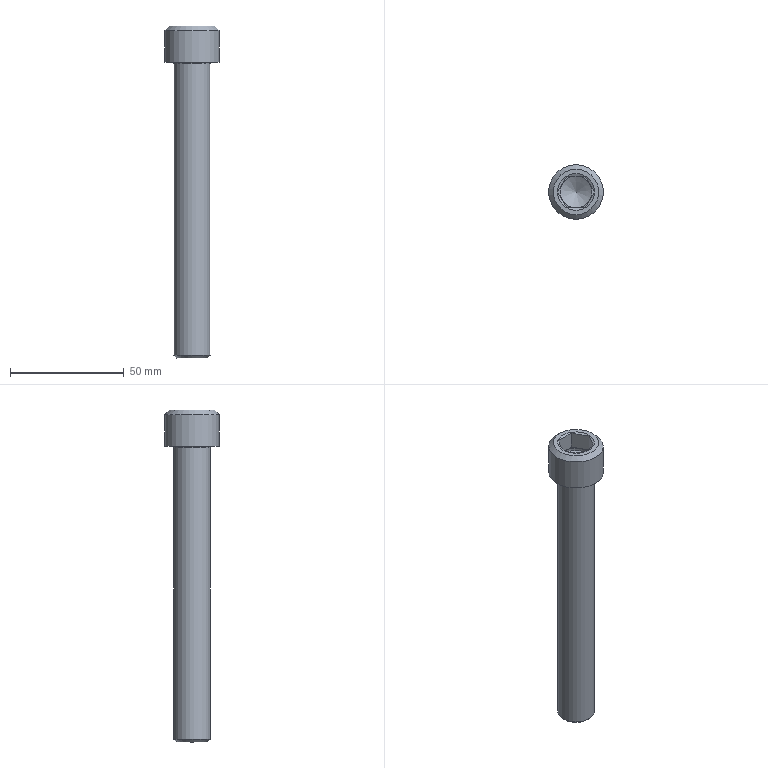Part | NX | features MAIN_BODY 2 | 1 solid | 20 faces | box 24 x 24 x 146 mm | volume 31440 mm3 | plane 11 | cone 5 | cylinder 3 | torus 1 | commonest cylinder face diameters 14 x1 16 x1 24 x1
STEP:
#1=CARTESIAN_POINT('',(635.,-653.001,267.));
#2=VERTEX_POINT('',#1);
#3=CARTESIAN_POINT('',(635.,-665.001,267.));
#4=DIRECTION('',(0.,0.,-1.));
#5=DIRECTION('',(0.,1.,0.));
#6=AXIS2_PLACEMENT_3D('',#3,#4,#5);
#7=CIRCLE('',#6,12.);
#8=EDGE_CURVE('',#2,#2,#7,.F.);
#9=ORIENTED_EDGE('',*,*,#8,.F.);
#10=EDGE_LOOP('',(#9));
#11=FACE_BOUND('',#10,.T.);
#12=CARTESIAN_POINT('',(635.,-677.001,253.));
#13=VERTEX_POINT('',#12);
#14=CARTESIAN_POINT('',(635.,-665.001,253.));
#15=DIRECTION('',(0.,0.,1.));
#16=DIRECTION('',(0.,-1.,0.));
#17=AXIS2_PLACEMENT_3D('',#14,#15,#16);
#18=CIRCLE('',#17,12.);
#19=EDGE_CURVE('',#13,#13,#18,.T.);
#20=ORIENTED_EDGE('',*,*,#19,.T.);
#21=EDGE_LOOP('',(#20));
#22=FACE_BOUND('',#21,.T.);
#23=CARTESIAN_POINT('',(635.,-665.001,261.));
#24=DIRECTION('',(0.,0.,1.));
#25=DIRECTION('',(0.,1.,0.));
#26=AXIS2_PLACEMENT_3D('',#23,#24,#25);
#27=CYLINDRICAL_SURFACE('',#26,12.);
#28=ADVANCED_FACE('',(#11,#22),#27,.T.);
#29=CARTESIAN_POINT('',(643.1,-665.001,269.));
#30=VERTEX_POINT('',#29);
#31=CARTESIAN_POINT('',(626.9,-665.001,269.));
#32=VERTEX_POINT('',#31);
#33=CARTESIAN_POINT('',(635.,-665.001,269.));
#34=DIRECTION('',(0.,0.,-1.));
#35=DIRECTION('',(0.,1.,0.));
#36=AXIS2_PLACEMENT_3D('',#33,#34,#35);
#37=CIRCLE('',#36,8.1);
#38=EDGE_CURVE('',#30,#32,#37,.T.);
#39=ORIENTED_EDGE('',*,*,#38,.T.);
#40=CARTESIAN_POINT('',(635.,-665.001,269.));
#41=DIRECTION('',(0.,0.,1.));
#42=DIRECTION('',(0.,-1.,0.));
#43=AXIS2_PLACEMENT_3D('',#40,#41,#42);
#44=CIRCLE('',#43,8.1);
#45=EDGE_CURVE('',#30,#32,#44,.T.);
#46=ORIENTED_EDGE('',*,*,#45,.F.);
#47=EDGE_LOOP('',(#39,#46));
#48=FACE_BOUND('',#47,.T.);
#49=CARTESIAN_POINT('',(635.,-655.001,269.));
#50=VERTEX_POINT('',#49);
#51=CARTESIAN_POINT('',(635.,-665.001,269.));
#52=DIRECTION('',(0.,0.,-1.));
#53=DIRECTION('',(0.,1.,0.));
#54=AXIS2_PLACEMENT_3D('',#51,#52,#53);
#55=CIRCLE('',#54,10.);
#56=EDGE_CURVE('',#50,#50,#55,.T.);
#57=ORIENTED_EDGE('',*,*,#56,.F.);
#58=EDGE_LOOP('',(#57));
#59=FACE_BOUND('',#58,.T.);
#60=CARTESIAN_POINT('',(635.,-665.001,269.));
#61=DIRECTION('',(0.,0.,1.));
#62=DIRECTION('',(0.,1.,0.));
#63=AXIS2_PLACEMENT_3D('',#60,#61,#62);
#64=PLANE('',#63);
#65=ADVANCED_FACE('',(#48,#59),#64,.T.);
#66=CARTESIAN_POINT('',(635.,-673.601,253.));
#67=VERTEX_POINT('',#66);
#68=CARTESIAN_POINT('',(635.,-665.001,253.));
#69=DIRECTION('',(0.,0.,1.));
#70=DIRECTION('',(0.,-1.,0.));
#71=AXIS2_PLACEMENT_3D('',#68,#69,#70);
#72=CIRCLE('',#71,8.6);
#73=EDGE_CURVE('',#67,#67,#72,.F.);
#74=ORIENTED_EDGE('',*,*,#73,.F.);
#75=EDGE_LOOP('',(#74));
#76=FACE_BOUND('',#75,.T.);
#77=ORIENTED_EDGE('',*,*,#19,.F.);
#78=EDGE_LOOP('',(#77));
#79=FACE_BOUND('',#78,.T.);
#80=CARTESIAN_POINT('',(635.,-665.001,253.));
#81=DIRECTION('',(0.,0.,-1.));
#82=DIRECTION('',(0.,-1.,0.));
#83=AXIS2_PLACEMENT_3D('',#80,#81,#82);
#84=PLANE('',#83);
#85=ADVANCED_FACE('',(#76,#79),#84,.T.);
#86=CARTESIAN_POINT('',(635.,-671.801,123.));
#87=VERTEX_POINT('',#86);
#88=CARTESIAN_POINT('',(635.,-665.001,123.));
#89=DIRECTION('',(0.,0.,1.));
#90=DIRECTION('',(0.,-1.,0.));
#91=AXIS2_PLACEMENT_3D('',#88,#89,#90);
#92=CIRCLE('',#91,6.8);
#93=EDGE_CURVE('',#87,#87,#92,.T.);
#94=ORIENTED_EDGE('',*,*,#93,.F.);
#95=EDGE_LOOP('',(#94));
#96=FACE_BOUND('',#95,.T.);
#97=CARTESIAN_POINT('',(635.,-665.001,123.));
#98=DIRECTION('',(0.,0.,-1.));
#99=DIRECTION('',(0.,-1.,0.));
#100=AXIS2_PLACEMENT_3D('',#97,#98,#99);
#101=PLANE('',#100);
#102=ADVANCED_FACE('',(#96),#101,.T.);
#103=CARTESIAN_POINT('',(635.,-673.001,252.4));
#104=VERTEX_POINT('',#103);
#105=CARTESIAN_POINT('',(635.,-665.001,252.4));
#106=DIRECTION('',(0.,0.,1.));
#107=DIRECTION('',(0.,-1.,0.));
#108=AXIS2_PLACEMENT_3D('',#105,#106,#107);
#109=CIRCLE('',#108,8.);
#110=EDGE_CURVE('',#104,#104,#109,.T.);
#111=ORIENTED_EDGE('',*,*,#110,.F.);
#112=EDGE_LOOP('',(#111));
#113=FACE_BOUND('',#112,.T.);
#114=CARTESIAN_POINT('',(635.,-673.001,124.2));
#115=VERTEX_POINT('',#114);
#116=CARTESIAN_POINT('',(635.,-665.001,124.2));
#117=DIRECTION('',(0.,0.,1.));
#118=DIRECTION('',(0.,-1.,0.));
#119=AXIS2_PLACEMENT_3D('',#116,#117,#118);
#120=CIRCLE('',#119,8.);
#121=EDGE_CURVE('',#115,#115,#120,.F.);
#122=ORIENTED_EDGE('',*,*,#121,.F.);
#123=EDGE_LOOP('',(#122));
#124=FACE_BOUND('',#123,.T.);
#125=CARTESIAN_POINT('',(635.,-665.001,253.));
#126=DIRECTION('',(0.,0.,-1.));
#127=DIRECTION('',(0.,-1.,0.));
#128=AXIS2_PLACEMENT_3D('',#125,#126,#127);
#129=CYLINDRICAL_SURFACE('',#128,8.);
#130=ADVANCED_FACE('',(#113,#124),#129,.T.);
#131=ORIENTED_EDGE('',*,*,#121,.T.);
#132=EDGE_LOOP('',(#131));
#133=FACE_BOUND('',#132,.T.);
#134=ORIENTED_EDGE('',*,*,#93,.T.);
#135=EDGE_LOOP('',(#134));
#136=FACE_BOUND('',#135,.T.);
#137=CARTESIAN_POINT('',(635.,-665.001,123.));
#138=DIRECTION('',(0.,0.,1.));
#139=DIRECTION('',(0.,1.,0.));
#140=AXIS2_PLACEMENT_3D('',#137,#138,#139);
#141=CONICAL_SURFACE('',#140,6.8,0.7854);
#142=ADVANCED_FACE('',(#133,#136),#141,.T.);
#143=ORIENTED_EDGE('',*,*,#8,.T.);
#144=EDGE_LOOP('',(#143));
#145=FACE_BOUND('',#144,.T.);
#146=ORIENTED_EDGE('',*,*,#56,.T.);
#147=EDGE_LOOP('',(#146));
#148=FACE_BOUND('',#147,.T.);
#149=CARTESIAN_POINT('',(635.,-665.001,269.));
#150=DIRECTION('',(0.,0.,-1.));
#151=DIRECTION('',(0.,-1.,0.));
#152=AXIS2_PLACEMENT_3D('',#149,#150,#151);
#153=CONICAL_SURFACE('',#152,10.,0.7854);
#154=ADVANCED_FACE('',(#145,#148),#153,.T.);
#155=ORIENTED_EDGE('',*,*,#73,.T.);
#156=EDGE_LOOP('',(#155));
#157=FACE_BOUND('',#156,.T.);
#158=ORIENTED_EDGE('',*,*,#110,.T.);
#159=EDGE_LOOP('',(#158));
#160=FACE_BOUND('',#159,.T.);
#161=CARTESIAN_POINT('',(635.,-665.001,252.4));
#162=DIRECTION('',(0.,0.,-1.));
#163=DIRECTION('',(0.,-1.,0.));
#164=AXIS2_PLACEMENT_3D('',#161,#162,#163);
#165=TOROIDAL_SURFACE('',#164,8.6,0.6);
#166=ADVANCED_FACE('',(#157,#160),#165,.F.);
#167=CARTESIAN_POINT('',(630.941,-658.001,268.995));
#168=VERTEX_POINT('',#167);
#169=CARTESIAN_POINT('',(626.9,-665.001,269.));
#170=CARTESIAN_POINT('',(627.56,-663.858,268.619));
#171=CARTESIAN_POINT('',(628.913,-661.514,268.13));
#172=CARTESIAN_POINT('',(630.281,-659.146,268.615));
#173=CARTESIAN_POINT('',(630.941,-658.001,268.995));
#174=B_SPLINE_CURVE_WITH_KNOTS('',3,(#169,#170,#171,#172,#173),.UNSPECIFIED.,.F.,.F.,(4,1,4),(0.000000238,0.004082,0.008163),.UNSPECIFIED.);
#175=EDGE_CURVE('',#32,#168,#174,.T.);
#176=ORIENTED_EDGE('',*,*,#175,.T.);
#177=CARTESIAN_POINT('',(639.059,-658.001,268.995));
#178=VERTEX_POINT('',#177);
#179=CARTESIAN_POINT('',(630.941,-658.001,268.995));
#180=CARTESIAN_POINT('',(632.26,-658.001,268.613));
#181=CARTESIAN_POINT('',(634.999,-658.001,268.116));
#182=CARTESIAN_POINT('',(637.747,-658.001,268.615));
#183=CARTESIAN_POINT('',(639.059,-658.001,268.995));
#184=B_SPLINE_CURVE_WITH_KNOTS('',3,(#179,#180,#181,#182,#183),.UNSPECIFIED.,.F.,.F.,(4,1,4),(0.00695,0.01105,0.01516),.UNSPECIFIED.);
#185=EDGE_CURVE('',#168,#178,#184,.T.);
#186=ORIENTED_EDGE('',*,*,#185,.T.);
#187=CARTESIAN_POINT('',(639.059,-658.001,268.995));
#188=CARTESIAN_POINT('',(639.719,-659.144,268.615));
#189=CARTESIAN_POINT('',(641.072,-661.488,268.13));
#190=CARTESIAN_POINT('',(642.439,-663.857,268.619));
#191=CARTESIAN_POINT('',(643.1,-665.001,269.));
#192=B_SPLINE_CURVE_WITH_KNOTS('',3,(#187,#188,#189,#190,#191),.UNSPECIFIED.,.F.,.F.,(4,1,4),(0.000000238,0.004082,0.008163),.UNSPECIFIED.);
#193=EDGE_CURVE('',#178,#30,#192,.T.);
#194=ORIENTED_EDGE('',*,*,#193,.T.);
#195=ORIENTED_EDGE('',*,*,#45,.T.);
#196=EDGE_LOOP('',(#176,#186,#194,#195));
#197=FACE_BOUND('',#196,.T.);
#198=CARTESIAN_POINT('',(635.,-665.001,264.323));
#199=DIRECTION('',(0.,0.,1.));
#200=DIRECTION('',(0.,1.,0.));
#201=AXIS2_PLACEMENT_3D('',#198,#199,#200);
#202=CONICAL_SURFACE('',#201,0.,1.047);
#203=ADVANCED_FACE('',(#197),#202,.F.);
#204=CARTESIAN_POINT('',(639.059,-672.001,268.995));
#205=VERTEX_POINT('',#204);
#206=CARTESIAN_POINT('',(630.941,-672.001,268.995));
#207=VERTEX_POINT('',#206);
#208=CARTESIAN_POINT('',(630.941,-672.001,268.995));
#209=CARTESIAN_POINT('',(632.26,-672.001,268.613));
#210=CARTESIAN_POINT('',(634.999,-672.001,268.116));
#211=CARTESIAN_POINT('',(637.747,-672.001,268.615));
#212=CARTESIAN_POINT('',(639.059,-672.001,268.995));
#213=B_SPLINE_CURVE_WITH_KNOTS('',3,(#208,#209,#210,#211,#212),.UNSPECIFIED.,.F.,.F.,(4,1,4),(0.00695,0.01105,0.01516),.UNSPECIFIED.);
#214=EDGE_CURVE('',#205,#207,#213,.F.);
#215=ORIENTED_EDGE('',*,*,#214,.T.);
#216=CARTESIAN_POINT('',(630.941,-672.001,268.995));
#217=CARTESIAN_POINT('',(630.281,-670.858,268.615));
#218=CARTESIAN_POINT('',(628.928,-668.513,268.13));
#219=CARTESIAN_POINT('',(627.561,-666.145,268.619));
#220=CARTESIAN_POINT('',(626.9,-665.001,269.));
#221=B_SPLINE_CURVE_WITH_KNOTS('',3,(#216,#217,#218,#219,#220),.UNSPECIFIED.,.F.,.F.,(4,1,4),(0.000000238,0.004082,0.008163),.UNSPECIFIED.);
#222=EDGE_CURVE('',#207,#32,#221,.T.);
#223=ORIENTED_EDGE('',*,*,#222,.T.);
#224=ORIENTED_EDGE('',*,*,#38,.F.);
#225=CARTESIAN_POINT('',(639.059,-672.001,268.995));
#226=CARTESIAN_POINT('',(639.719,-670.858,268.615));
#227=CARTESIAN_POINT('',(641.072,-668.513,268.13));
#228=CARTESIAN_POINT('',(642.439,-666.145,268.619));
#229=CARTESIAN_POINT('',(643.1,-665.001,269.));
#230=B_SPLINE_CURVE_WITH_KNOTS('',3,(#225,#226,#227,#228,#229),.UNSPECIFIED.,.F.,.F.,(4,1,4),(0.000000238,0.004082,0.008163),.UNSPECIFIED.);
#231=EDGE_CURVE('',#205,#30,#230,.T.);
#232=ORIENTED_EDGE('',*,*,#231,.F.);
#233=EDGE_LOOP('',(#215,#223,#224,#232));
#234=FACE_BOUND('',#233,.T.);
#235=CARTESIAN_POINT('',(635.,-665.001,264.323));
#236=DIRECTION('',(0.,0.,1.));
#237=DIRECTION('',(0.,1.,0.));
#238=AXIS2_PLACEMENT_3D('',#235,#236,#237);
#239=CONICAL_SURFACE('',#238,0.,1.047);
#240=ADVANCED_FACE('',(#234),#239,.F.);
#241=CARTESIAN_POINT('',(635.,-672.001,259.8));
#242=VERTEX_POINT('',#241);
#243=CARTESIAN_POINT('',(635.,-665.001,259.8));
#244=DIRECTION('',(0.,0.,1.));
#245=DIRECTION('',(0.,-1.,0.));
#246=AXIS2_PLACEMENT_3D('',#243,#244,#245);
#247=CIRCLE('',#246,7.);
#248=EDGE_CURVE('',#242,#242,#247,.T.);
#249=ORIENTED_EDGE('',*,*,#248,.T.);
#250=EDGE_LOOP('',(#249));
#251=FACE_BOUND('',#250,.T.);
#252=CARTESIAN_POINT('',(635.,-665.001,255.759));
#253=VERTEX_POINT('',#252);
#254=VERTEX_LOOP('',#253);
#255=FACE_BOUND('',#254,.T.);
#256=CARTESIAN_POINT('',(635.,-665.001,259.8));
#257=DIRECTION('',(0.,0.,1.));
#258=DIRECTION('',(0.,1.,0.));
#259=AXIS2_PLACEMENT_3D('',#256,#257,#258);
#260=CONICAL_SURFACE('',#259,7.,1.047);
#261=ADVANCED_FACE('',(#251,#255),#260,.F.);
#262=ORIENTED_EDGE('',*,*,#248,.F.);
#263=EDGE_LOOP('',(#262));
#264=FACE_BOUND('',#263,.T.);
#265=CARTESIAN_POINT('',(635.,-672.001,261.));
#266=VERTEX_POINT('',#265);
#267=CARTESIAN_POINT('',(635.,-658.001,261.));
#268=VERTEX_POINT('',#267);
#269=CARTESIAN_POINT('',(635.,-665.001,261.));
#270=DIRECTION('',(0.,0.,1.));
#271=DIRECTION('',(0.,-1.,0.));
#272=AXIS2_PLACEMENT_3D('',#269,#270,#271);
#273=CIRCLE('',#272,7.);
#274=EDGE_CURVE('',#266,#268,#273,.T.);
#275=ORIENTED_EDGE('',*,*,#274,.T.);
#276=CARTESIAN_POINT('',(635.,-665.001,261.));
#277=DIRECTION('',(0.,0.,1.));
#278=DIRECTION('',(0.,-1.,0.));
#279=AXIS2_PLACEMENT_3D('',#276,#277,#278);
#280=CIRCLE('',#279,7.);
#281=EDGE_CURVE('',#268,#266,#280,.T.);
#282=ORIENTED_EDGE('',*,*,#281,.T.);
#283=EDGE_LOOP('',(#275,#282));
#284=FACE_BOUND('',#283,.T.);
#285=CARTESIAN_POINT('',(635.,-665.001,261.));
#286=DIRECTION('',(0.,0.,-1.));
#287=DIRECTION('',(0.,-1.,0.));
#288=AXIS2_PLACEMENT_3D('',#285,#286,#287);
#289=CYLINDRICAL_SURFACE('',#288,7.);
#290=ADVANCED_FACE('',(#264,#284),#289,.F.);
#291=CARTESIAN_POINT('',(630.941,-658.001,261.));
#292=VERTEX_POINT('',#291);
#293=CARTESIAN_POINT('',(630.941,-658.001,261.));
#294=DIRECTION('',(1.,0.,0.));
#295=VECTOR('',#294,1000.);
#296=LINE('',#293,#295);
#297=EDGE_CURVE('',#292,#268,#296,.T.);
#298=ORIENTED_EDGE('',*,*,#297,.F.);
#299=CARTESIAN_POINT('',(626.9,-665.001,261.));
#300=VERTEX_POINT('',#299);
#301=CARTESIAN_POINT('',(626.9,-665.001,261.));
#302=DIRECTION('',(0.5,0.866,0.));
#303=VECTOR('',#302,1000.);
#304=LINE('',#301,#303);
#305=EDGE_CURVE('',#300,#292,#304,.T.);
#306=ORIENTED_EDGE('',*,*,#305,.F.);
#307=CARTESIAN_POINT('',(630.941,-672.001,261.));
#308=VERTEX_POINT('',#307);
#309=CARTESIAN_POINT('',(630.941,-672.001,261.));
#310=DIRECTION('',(-0.5,0.866,0.));
#311=VECTOR('',#310,1000.);
#312=LINE('',#309,#311);
#313=EDGE_CURVE('',#308,#300,#312,.T.);
#314=ORIENTED_EDGE('',*,*,#313,.F.);
#315=CARTESIAN_POINT('',(639.059,-672.001,261.));
#316=DIRECTION('',(-1.,0.,0.));
#317=VECTOR('',#316,1000.);
#318=LINE('',#315,#317);
#319=EDGE_CURVE('',#266,#308,#318,.T.);
#320=ORIENTED_EDGE('',*,*,#319,.F.);
#321=ORIENTED_EDGE('',*,*,#281,.F.);
#322=EDGE_LOOP('',(#298,#306,#314,#320,#321));
#323=FACE_BOUND('',#322,.T.);
#324=CARTESIAN_POINT('',(635.,-665.001,261.));
#325=DIRECTION('',(0.,0.,1.));
#326=DIRECTION('',(0.,1.,0.));
#327=AXIS2_PLACEMENT_3D('',#324,#325,#326);
#328=PLANE('',#327);
#329=ADVANCED_FACE('',(#323),#328,.T.);
#330=CARTESIAN_POINT('',(639.059,-672.001,261.));
#331=VERTEX_POINT('',#330);
#332=CARTESIAN_POINT('',(639.059,-672.001,261.));
#333=DIRECTION('',(-1.,0.,0.));
#334=VECTOR('',#333,1000.);
#335=LINE('',#332,#334);
#336=EDGE_CURVE('',#331,#266,#335,.T.);
#337=ORIENTED_EDGE('',*,*,#336,.F.);
#338=CARTESIAN_POINT('',(643.1,-665.001,261.));
#339=VERTEX_POINT('',#338);
#340=CARTESIAN_POINT('',(639.059,-672.001,261.));
#341=DIRECTION('',(0.5,0.866,0.));
#342=VECTOR('',#341,1000.);
#343=LINE('',#340,#342);
#344=EDGE_CURVE('',#331,#339,#343,.T.);
#345=ORIENTED_EDGE('',*,*,#344,.T.);
#346=CARTESIAN_POINT('',(639.059,-658.001,261.));
#347=VERTEX_POINT('',#346);
#348=CARTESIAN_POINT('',(639.059,-658.001,261.));
#349=DIRECTION('',(0.5,-0.866,0.));
#350=VECTOR('',#349,1000.);
#351=LINE('',#348,#350);
#352=EDGE_CURVE('',#347,#339,#351,.T.);
#353=ORIENTED_EDGE('',*,*,#352,.F.);
#354=CARTESIAN_POINT('',(630.941,-658.001,261.));
#355=DIRECTION('',(1.,0.,0.));
#356=VECTOR('',#355,1000.);
#357=LINE('',#354,#356);
#358=EDGE_CURVE('',#268,#347,#357,.T.);
#359=ORIENTED_EDGE('',*,*,#358,.F.);
#360=ORIENTED_EDGE('',*,*,#274,.F.);
#361=EDGE_LOOP('',(#337,#345,#353,#359,#360));
#362=FACE_BOUND('',#361,.T.);
#363=CARTESIAN_POINT('',(635.,-665.001,261.));
#364=DIRECTION('',(0.,0.,1.));
#365=DIRECTION('',(0.,1.,0.));
#366=AXIS2_PLACEMENT_3D('',#363,#364,#365);
#367=PLANE('',#366);
#368=ADVANCED_FACE('',(#362),#367,.T.);
#369=CARTESIAN_POINT('',(639.059,-658.001,261.));
#370=DIRECTION('',(0.,0.,1.));
#371=VECTOR('',#370,1000.);
#372=LINE('',#369,#371);
#373=EDGE_CURVE('',#347,#178,#372,.T.);
#374=ORIENTED_EDGE('',*,*,#373,.F.);
#375=ORIENTED_EDGE('',*,*,#352,.T.);
#376=CARTESIAN_POINT('',(643.1,-665.001,261.));
#377=DIRECTION('',(0.,0.,1.));
#378=VECTOR('',#377,1000.);
#379=LINE('',#376,#378);
#380=EDGE_CURVE('',#339,#30,#379,.T.);
#381=ORIENTED_EDGE('',*,*,#380,.T.);
#382=ORIENTED_EDGE('',*,*,#193,.F.);
#383=EDGE_LOOP('',(#374,#375,#381,#382));
#384=FACE_BOUND('',#383,.T.);
#385=CARTESIAN_POINT('',(639.059,-658.001,261.));
#386=DIRECTION('',(0.866,0.5,0.));
#387=DIRECTION('',(0.5,-0.866,0.));
#388=AXIS2_PLACEMENT_3D('',#385,#386,#387);
#389=PLANE('',#388);
#390=ADVANCED_FACE('',(#384),#389,.F.);
#391=ORIENTED_EDGE('',*,*,#231,.T.);
#392=ORIENTED_EDGE('',*,*,#380,.F.);
#393=ORIENTED_EDGE('',*,*,#344,.F.);
#394=CARTESIAN_POINT('',(639.059,-672.001,261.));
#395=DIRECTION('',(0.,0.,1.));
#396=VECTOR('',#395,1000.);
#397=LINE('',#394,#396);
#398=EDGE_CURVE('',#331,#205,#397,.T.);
#399=ORIENTED_EDGE('',*,*,#398,.T.);
#400=EDGE_LOOP('',(#391,#392,#393,#399));
#401=FACE_BOUND('',#400,.T.);
#402=CARTESIAN_POINT('',(639.059,-672.001,261.));
#403=DIRECTION('',(-0.866,0.5,0.));
#404=DIRECTION('',(0.5,0.866,0.));
#405=AXIS2_PLACEMENT_3D('',#402,#403,#404);
#406=PLANE('',#405);
#407=ADVANCED_FACE('',(#401),#406,.T.);
#408=ORIENTED_EDGE('',*,*,#398,.F.);
#409=ORIENTED_EDGE('',*,*,#336,.T.);
#410=ORIENTED_EDGE('',*,*,#319,.T.);
#411=CARTESIAN_POINT('',(630.941,-672.001,261.));
#412=DIRECTION('',(0.,0.,1.));
#413=VECTOR('',#412,1000.);
#414=LINE('',#411,#413);
#415=EDGE_CURVE('',#308,#207,#414,.T.);
#416=ORIENTED_EDGE('',*,*,#415,.T.);
#417=ORIENTED_EDGE('',*,*,#214,.F.);
#418=EDGE_LOOP('',(#408,#409,#410,#416,#417));
#419=FACE_BOUND('',#418,.T.);
#420=CARTESIAN_POINT('',(639.059,-672.001,261.));
#421=DIRECTION('',(0.,-1.,0.));
#422=DIRECTION('',(-1.,0.,0.));
#423=AXIS2_PLACEMENT_3D('',#420,#421,#422);
#424=PLANE('',#423);
#425=ADVANCED_FACE('',(#419),#424,.F.);
#426=ORIENTED_EDGE('',*,*,#415,.F.);
#427=ORIENTED_EDGE('',*,*,#313,.T.);
#428=CARTESIAN_POINT('',(626.9,-665.001,261.));
#429=DIRECTION('',(0.,0.,1.));
#430=VECTOR('',#429,1000.);
#431=LINE('',#428,#430);
#432=EDGE_CURVE('',#300,#32,#431,.T.);
#433=ORIENTED_EDGE('',*,*,#432,.T.);
#434=ORIENTED_EDGE('',*,*,#222,.F.);
#435=EDGE_LOOP('',(#426,#427,#433,#434));
#436=FACE_BOUND('',#435,.T.);
#437=CARTESIAN_POINT('',(630.941,-672.001,261.));
#438=DIRECTION('',(-0.866,-0.5,0.));
#439=DIRECTION('',(-0.5,0.866,0.));
#440=AXIS2_PLACEMENT_3D('',#437,#438,#439);
#441=PLANE('',#440);
#442=ADVANCED_FACE('',(#436),#441,.F.);
#443=ORIENTED_EDGE('',*,*,#432,.F.);
#444=ORIENTED_EDGE('',*,*,#305,.T.);
#445=CARTESIAN_POINT('',(630.941,-658.001,261.));
#446=DIRECTION('',(0.,0.,1.));
#447=VECTOR('',#446,1000.);
#448=LINE('',#445,#447);
#449=EDGE_CURVE('',#292,#168,#448,.T.);
#450=ORIENTED_EDGE('',*,*,#449,.T.);
#451=ORIENTED_EDGE('',*,*,#175,.F.);
#452=EDGE_LOOP('',(#443,#444,#450,#451));
#453=FACE_BOUND('',#452,.T.);
#454=CARTESIAN_POINT('',(626.9,-665.001,261.));
#455=DIRECTION('',(-0.866,0.5,0.));
#456=DIRECTION('',(0.5,0.866,0.));
#457=AXIS2_PLACEMENT_3D('',#454,#455,#456);
#458=PLANE('',#457);
#459=ADVANCED_FACE('',(#453),#458,.F.);
#460=ORIENTED_EDGE('',*,*,#449,.F.);
#461=ORIENTED_EDGE('',*,*,#297,.T.);
#462=ORIENTED_EDGE('',*,*,#358,.T.);
#463=ORIENTED_EDGE('',*,*,#373,.T.);
#464=ORIENTED_EDGE('',*,*,#185,.F.);
#465=EDGE_LOOP('',(#460,#461,#462,#463,#464));
#466=FACE_BOUND('',#465,.T.);
#467=CARTESIAN_POINT('',(630.941,-658.001,261.));
#468=DIRECTION('',(0.,1.,0.));
#469=DIRECTION('',(0.,0.,-1.));
#470=AXIS2_PLACEMENT_3D('',#467,#468,#469);
#471=PLANE('',#470);
#472=ADVANCED_FACE('',(#466),#471,.F.);
#473=CLOSED_SHELL('',(#28,#65,#85,#102,#130,#142,#154,#166,#203,#240,#261,#290,#329,#368,#390,#407,#425,#442,#459,#472));
#474=MANIFOLD_SOLID_BREP('',#473);
#475=(LENGTH_UNIT()NAMED_UNIT(*)SI_UNIT(.MILLI.,.METRE.));
#476=UNCERTAINTY_MEASURE_WITH_UNIT(LENGTH_MEASURE(0.0508),#475,'','');
#477=(NAMED_UNIT(*)PLANE_ANGLE_UNIT()SI_UNIT($,.RADIAN.));
#478=(NAMED_UNIT(*)SI_UNIT($,.STERADIAN.)SOLID_ANGLE_UNIT());
#479=(GEOMETRIC_REPRESENTATION_CONTEXT(3)GLOBAL_UNCERTAINTY_ASSIGNED_CONTEXT((#476))GLOBAL_UNIT_ASSIGNED_CONTEXT((#475,#477,#478))REPRESENTATION_CONTEXT('',''));
#480=ADVANCED_BREP_SHAPE_REPRESENTATION('',(#474),#479);